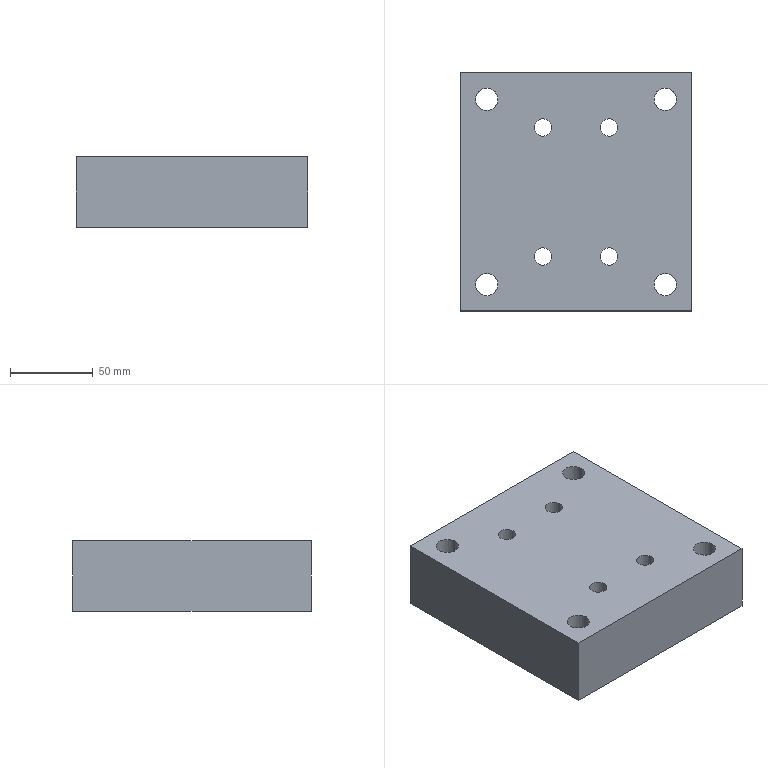Part | STEP file | lll_id2202_x_t | 1 solid | 44 faces | box 140 x 144 x 42.5 mm | volume 713752 mm3 | cylinder 22 | plane 20 | cone 2 | commonest cylinder face diameters 10 x8 10.506 x4 13.509 x4 20.007 x4 10.505 x2
STEP:
#1=CARTESIAN_POINT('',(1650.253,39.,152.5));
#2=VERTEX_POINT('',#1);
#3=CARTESIAN_POINT('',(1645.,39.,152.5));
#4=DIRECTION('',(0.,0.,1.));
#5=DIRECTION('',(1.,0.,0.));
#6=AXIS2_PLACEMENT_3D('',#3,#4,#5);
#7=CIRCLE('',#6,5.253);
#8=EDGE_CURVE('',#2,#2,#7,.T.);
#9=ORIENTED_EDGE('',*,*,#8,.F.);
#10=EDGE_LOOP('',(#9));
#11=FACE_BOUND('',#10,.T.);
#12=CARTESIAN_POINT('',(1610.253,39.,152.5));
#13=VERTEX_POINT('',#12);
#14=CARTESIAN_POINT('',(1605.,39.,152.5));
#15=DIRECTION('',(0.,0.,1.));
#16=DIRECTION('',(1.,0.,0.));
#17=AXIS2_PLACEMENT_3D('',#14,#15,#16);
#18=CIRCLE('',#17,5.253);
#19=EDGE_CURVE('',#13,#13,#18,.T.);
#20=ORIENTED_EDGE('',*,*,#19,.F.);
#21=EDGE_LOOP('',(#20));
#22=FACE_BOUND('',#21,.T.);
#23=CARTESIAN_POINT('',(1610.253,-39.,152.5));
#24=VERTEX_POINT('',#23);
#25=CARTESIAN_POINT('',(1605.,-39.,152.5));
#26=DIRECTION('',(0.,0.,1.));
#27=DIRECTION('',(1.,0.,0.));
#28=AXIS2_PLACEMENT_3D('',#25,#26,#27);
#29=CIRCLE('',#28,5.253);
#30=EDGE_CURVE('',#24,#24,#29,.T.);
#31=ORIENTED_EDGE('',*,*,#30,.F.);
#32=EDGE_LOOP('',(#31));
#33=FACE_BOUND('',#32,.T.);
#34=CARTESIAN_POINT('',(1650.253,-39.,152.5));
#35=VERTEX_POINT('',#34);
#36=CARTESIAN_POINT('',(1645.,-39.,152.5));
#37=DIRECTION('',(0.,0.,1.));
#38=DIRECTION('',(1.,0.,0.));
#39=AXIS2_PLACEMENT_3D('',#36,#37,#38);
#40=CIRCLE('',#39,5.253);
#41=EDGE_CURVE('',#35,#35,#40,.T.);
#42=ORIENTED_EDGE('',*,*,#41,.F.);
#43=EDGE_LOOP('',(#42));
#44=FACE_BOUND('',#43,.T.);
#45=CARTESIAN_POINT('',(1685.755,56.,152.5));
#46=VERTEX_POINT('',#45);
#47=CARTESIAN_POINT('',(1679.,56.,152.5));
#48=DIRECTION('',(0.,0.,1.));
#49=DIRECTION('',(1.,0.,0.));
#50=AXIS2_PLACEMENT_3D('',#47,#48,#49);
#51=CIRCLE('',#50,6.755);
#52=EDGE_CURVE('',#46,#46,#51,.T.);
#53=ORIENTED_EDGE('',*,*,#52,.F.);
#54=EDGE_LOOP('',(#53));
#55=FACE_BOUND('',#54,.T.);
#56=CARTESIAN_POINT('',(1577.755,56.,152.5));
#57=VERTEX_POINT('',#56);
#58=CARTESIAN_POINT('',(1571.,56.,152.5));
#59=DIRECTION('',(0.,0.,1.));
#60=DIRECTION('',(1.,0.,0.));
#61=AXIS2_PLACEMENT_3D('',#58,#59,#60);
#62=CIRCLE('',#61,6.755);
#63=EDGE_CURVE('',#57,#57,#62,.T.);
#64=ORIENTED_EDGE('',*,*,#63,.F.);
#65=EDGE_LOOP('',(#64));
#66=FACE_BOUND('',#65,.T.);
#67=CARTESIAN_POINT('',(1577.755,-56.,152.5));
#68=VERTEX_POINT('',#67);
#69=CARTESIAN_POINT('',(1571.,-56.,152.5));
#70=DIRECTION('',(0.,0.,1.));
#71=DIRECTION('',(1.,0.,0.));
#72=AXIS2_PLACEMENT_3D('',#69,#70,#71);
#73=CIRCLE('',#72,6.755);
#74=EDGE_CURVE('',#68,#68,#73,.T.);
#75=ORIENTED_EDGE('',*,*,#74,.F.);
#76=EDGE_LOOP('',(#75));
#77=FACE_BOUND('',#76,.T.);
#78=CARTESIAN_POINT('',(1685.755,-56.,152.5));
#79=VERTEX_POINT('',#78);
#80=CARTESIAN_POINT('',(1679.,-56.,152.5));
#81=DIRECTION('',(0.,0.,1.));
#82=DIRECTION('',(1.,0.,0.));
#83=AXIS2_PLACEMENT_3D('',#80,#81,#82);
#84=CIRCLE('',#83,6.755);
#85=EDGE_CURVE('',#79,#79,#84,.T.);
#86=ORIENTED_EDGE('',*,*,#85,.F.);
#87=EDGE_LOOP('',(#86));
#88=FACE_BOUND('',#87,.T.);
#89=CARTESIAN_POINT('',(1695.,-72.,152.5));
#90=VERTEX_POINT('',#89);
#91=CARTESIAN_POINT('',(1555.,-72.,152.5));
#92=VERTEX_POINT('',#91);
#93=CARTESIAN_POINT('',(1625.,-72.,152.5));
#94=DIRECTION('',(-1.,0.,0.));
#95=VECTOR('',#94,1.);
#96=LINE('',#93,#95);
#97=EDGE_CURVE('',#90,#92,#96,.T.);
#98=ORIENTED_EDGE('',*,*,#97,.F.);
#99=CARTESIAN_POINT('',(1695.,72.,152.5));
#100=VERTEX_POINT('',#99);
#101=CARTESIAN_POINT('',(1695.,0.,152.5));
#102=DIRECTION('',(0.,-1.,0.));
#103=VECTOR('',#102,1.);
#104=LINE('',#101,#103);
#105=EDGE_CURVE('',#100,#90,#104,.T.);
#106=ORIENTED_EDGE('',*,*,#105,.F.);
#107=CARTESIAN_POINT('',(1555.,72.,152.5));
#108=VERTEX_POINT('',#107);
#109=CARTESIAN_POINT('',(1625.,72.,152.5));
#110=DIRECTION('',(1.,0.,0.));
#111=VECTOR('',#110,1.);
#112=LINE('',#109,#111);
#113=EDGE_CURVE('',#108,#100,#112,.T.);
#114=ORIENTED_EDGE('',*,*,#113,.F.);
#115=CARTESIAN_POINT('',(1555.,0.,152.5));
#116=DIRECTION('',(0.,1.,0.));
#117=VECTOR('',#116,1.);
#118=LINE('',#115,#117);
#119=EDGE_CURVE('',#92,#108,#118,.T.);
#120=ORIENTED_EDGE('',*,*,#119,.F.);
#121=EDGE_LOOP('',(#98,#106,#114,#120));
#122=FACE_BOUND('',#121,.T.);
#123=CARTESIAN_POINT('',(1625.,0.,152.5));
#124=DIRECTION('',(0.,0.,1.));
#125=DIRECTION('',(1.,0.,0.));
#126=AXIS2_PLACEMENT_3D('',#123,#124,#125);
#127=PLANE('',#126);
#128=ADVANCED_FACE('',(#11,#22,#33,#44,#55,#66,#77,#88,#122),#127,.T.);
#129=CARTESIAN_POINT('',(1695.,-72.,110.));
#130=VERTEX_POINT('',#129);
#131=CARTESIAN_POINT('',(1555.,-72.,110.));
#132=VERTEX_POINT('',#131);
#133=CARTESIAN_POINT('',(1625.,-72.,110.));
#134=DIRECTION('',(-1.,0.,0.));
#135=VECTOR('',#134,1.);
#136=LINE('',#133,#135);
#137=EDGE_CURVE('',#130,#132,#136,.T.);
#138=ORIENTED_EDGE('',*,*,#137,.F.);
#139=CARTESIAN_POINT('',(1695.,-72.,-23.));
#140=DIRECTION('',(0.,0.,1.));
#141=VECTOR('',#140,1.);
#142=LINE('',#139,#141);
#143=EDGE_CURVE('',#130,#90,#142,.T.);
#144=ORIENTED_EDGE('',*,*,#143,.T.);
#145=ORIENTED_EDGE('',*,*,#97,.T.);
#146=CARTESIAN_POINT('',(1555.,-72.,-23.));
#147=DIRECTION('',(0.,0.,1.));
#148=VECTOR('',#147,1.);
#149=LINE('',#146,#148);
#150=EDGE_CURVE('',#132,#92,#149,.T.);
#151=ORIENTED_EDGE('',*,*,#150,.F.);
#152=EDGE_LOOP('',(#138,#144,#145,#151));
#153=FACE_OUTER_BOUND('',#152,.T.);
#154=CARTESIAN_POINT('',(1625.,-72.,-23.));
#155=DIRECTION('',(0.,-1.,0.));
#156=DIRECTION('',(0.,0.,-1.));
#157=AXIS2_PLACEMENT_3D('',#154,#155,#156);
#158=PLANE('',#157);
#159=ADVANCED_FACE('',(#153),#158,.T.);
#160=CARTESIAN_POINT('',(1555.,72.,110.));
#161=VERTEX_POINT('',#160);
#162=CARTESIAN_POINT('',(1555.,0.,110.));
#163=DIRECTION('',(0.,-1.,0.));
#164=VECTOR('',#163,1.);
#165=LINE('',#162,#164);
#166=EDGE_CURVE('',#161,#132,#165,.T.);
#167=ORIENTED_EDGE('',*,*,#166,.T.);
#168=ORIENTED_EDGE('',*,*,#150,.T.);
#169=ORIENTED_EDGE('',*,*,#119,.T.);
#170=CARTESIAN_POINT('',(1555.,72.,-23.));
#171=DIRECTION('',(0.,0.,1.));
#172=VECTOR('',#171,1.);
#173=LINE('',#170,#172);
#174=EDGE_CURVE('',#161,#108,#173,.T.);
#175=ORIENTED_EDGE('',*,*,#174,.F.);
#176=EDGE_LOOP('',(#167,#168,#169,#175));
#177=FACE_OUTER_BOUND('',#176,.T.);
#178=CARTESIAN_POINT('',(1555.,0.,-23.));
#179=DIRECTION('',(-1.,0.,0.));
#180=DIRECTION('',(0.,0.,1.));
#181=AXIS2_PLACEMENT_3D('',#178,#179,#180);
#182=PLANE('',#181);
#183=ADVANCED_FACE('',(#177),#182,.T.);
#184=CARTESIAN_POINT('',(1695.,72.,110.));
#185=VERTEX_POINT('',#184);
#186=CARTESIAN_POINT('',(1625.,72.,110.));
#187=DIRECTION('',(1.,0.,0.));
#188=VECTOR('',#187,1.);
#189=LINE('',#186,#188);
#190=EDGE_CURVE('',#161,#185,#189,.T.);
#191=ORIENTED_EDGE('',*,*,#190,.F.);
#192=ORIENTED_EDGE('',*,*,#174,.T.);
#193=ORIENTED_EDGE('',*,*,#113,.T.);
#194=CARTESIAN_POINT('',(1695.,72.,-23.));
#195=DIRECTION('',(0.,0.,1.));
#196=VECTOR('',#195,1.);
#197=LINE('',#194,#196);
#198=EDGE_CURVE('',#185,#100,#197,.T.);
#199=ORIENTED_EDGE('',*,*,#198,.F.);
#200=EDGE_LOOP('',(#191,#192,#193,#199));
#201=FACE_OUTER_BOUND('',#200,.T.);
#202=CARTESIAN_POINT('',(1625.,72.,-23.));
#203=DIRECTION('',(0.,1.,0.));
#204=DIRECTION('',(0.,0.,1.));
#205=AXIS2_PLACEMENT_3D('',#202,#203,#204);
#206=PLANE('',#205);
#207=ADVANCED_FACE('',(#201),#206,.T.);
#208=CARTESIAN_POINT('',(1695.,0.,110.));
#209=DIRECTION('',(0.,-1.,0.));
#210=VECTOR('',#209,1.);
#211=LINE('',#208,#210);
#212=EDGE_CURVE('',#185,#130,#211,.T.);
#213=ORIENTED_EDGE('',*,*,#212,.F.);
#214=ORIENTED_EDGE('',*,*,#198,.T.);
#215=ORIENTED_EDGE('',*,*,#105,.T.);
#216=ORIENTED_EDGE('',*,*,#143,.F.);
#217=EDGE_LOOP('',(#213,#214,#215,#216));
#218=FACE_OUTER_BOUND('',#217,.T.);
#219=CARTESIAN_POINT('',(1695.,0.,-23.));
#220=DIRECTION('',(1.,0.,0.));
#221=DIRECTION('',(0.,0.,-1.));
#222=AXIS2_PLACEMENT_3D('',#219,#220,#221);
#223=PLANE('',#222);
#224=ADVANCED_FACE('',(#218),#223,.T.);
#225=CARTESIAN_POINT('',(1576.253,26.,110.));
#226=VERTEX_POINT('',#225);
#227=CARTESIAN_POINT('',(1571.,26.,110.));
#228=DIRECTION('',(0.,0.,1.));
#229=DIRECTION('',(1.,0.,0.));
#230=AXIS2_PLACEMENT_3D('',#227,#228,#229);
#231=CIRCLE('',#230,5.253);
#232=EDGE_CURVE('',#226,#226,#231,.T.);
#233=ORIENTED_EDGE('',*,*,#232,.T.);
#234=EDGE_LOOP('',(#233));
#235=FACE_BOUND('',#234,.T.);
#236=CARTESIAN_POINT('',(1689.004,56.,110.));
#237=VERTEX_POINT('',#236);
#238=CARTESIAN_POINT('',(1679.,56.,110.));
#239=DIRECTION('',(0.,0.,1.));
#240=DIRECTION('',(1.,0.,0.));
#241=AXIS2_PLACEMENT_3D('',#238,#239,#240);
#242=CIRCLE('',#241,10.004);
#243=EDGE_CURVE('',#237,#237,#242,.T.);
#244=ORIENTED_EDGE('',*,*,#243,.T.);
#245=EDGE_LOOP('',(#244));
#246=FACE_BOUND('',#245,.T.);
#247=CARTESIAN_POINT('',(1581.004,56.,110.));
#248=VERTEX_POINT('',#247);
#249=CARTESIAN_POINT('',(1571.,56.,110.));
#250=DIRECTION('',(0.,0.,1.));
#251=DIRECTION('',(1.,0.,0.));
#252=AXIS2_PLACEMENT_3D('',#249,#250,#251);
#253=CIRCLE('',#252,10.004);
#254=EDGE_CURVE('',#248,#248,#253,.T.);
#255=ORIENTED_EDGE('',*,*,#254,.T.);
#256=EDGE_LOOP('',(#255));
#257=FACE_BOUND('',#256,.T.);
#258=CARTESIAN_POINT('',(1581.004,-56.,110.));
#259=VERTEX_POINT('',#258);
#260=CARTESIAN_POINT('',(1571.,-56.,110.));
#261=DIRECTION('',(0.,0.,1.));
#262=DIRECTION('',(1.,0.,0.));
#263=AXIS2_PLACEMENT_3D('',#260,#261,#262);
#264=CIRCLE('',#263,10.004);
#265=EDGE_CURVE('',#259,#259,#264,.T.);
#266=ORIENTED_EDGE('',*,*,#265,.T.);
#267=EDGE_LOOP('',(#266));
#268=FACE_BOUND('',#267,.T.);
#269=CARTESIAN_POINT('',(1684.253,-26.,110.));
#270=VERTEX_POINT('',#269);
#271=CARTESIAN_POINT('',(1679.,-26.,110.));
#272=DIRECTION('',(0.,0.,1.));
#273=DIRECTION('',(1.,0.,0.));
#274=AXIS2_PLACEMENT_3D('',#271,#272,#273);
#275=CIRCLE('',#274,5.253);
#276=EDGE_CURVE('',#270,#270,#275,.T.);
#277=ORIENTED_EDGE('',*,*,#276,.T.);
#278=EDGE_LOOP('',(#277));
#279=FACE_BOUND('',#278,.T.);
#280=CARTESIAN_POINT('',(1689.004,-56.,110.));
#281=VERTEX_POINT('',#280);
#282=CARTESIAN_POINT('',(1679.,-56.,110.));
#283=DIRECTION('',(0.,0.,1.));
#284=DIRECTION('',(1.,0.,0.));
#285=AXIS2_PLACEMENT_3D('',#282,#283,#284);
#286=CIRCLE('',#285,10.004);
#287=EDGE_CURVE('',#281,#281,#286,.T.);
#288=ORIENTED_EDGE('',*,*,#287,.T.);
#289=EDGE_LOOP('',(#288));
#290=FACE_BOUND('',#289,.T.);
#291=CARTESIAN_POINT('',(1652.051,-11.,110.));
#292=VERTEX_POINT('',#291);
#293=CARTESIAN_POINT('',(1597.949,-11.,110.));
#294=VERTEX_POINT('',#293);
#295=CARTESIAN_POINT('',(2132.435,-11.,110.));
#296=DIRECTION('',(-1.,0.,0.));
#297=VECTOR('',#296,1.);
#298=LINE('',#295,#297);
#299=EDGE_CURVE('',#292,#294,#298,.T.);
#300=ORIENTED_EDGE('',*,*,#299,.T.);
#301=CARTESIAN_POINT('',(1590.,-16.752,110.));
#302=VERTEX_POINT('',#301);
#303=CARTESIAN_POINT('',(1593.408,-13.094,110.));
#304=DIRECTION('',(0.,0.,1.));
#305=DIRECTION('',(1.,0.,0.));
#306=AXIS2_PLACEMENT_3D('',#303,#304,#305);
#307=CIRCLE('',#306,5.);
#308=EDGE_CURVE('',#294,#302,#307,.T.);
#309=ORIENTED_EDGE('',*,*,#308,.T.);
#310=CARTESIAN_POINT('',(1590.,-48.248,110.));
#311=VERTEX_POINT('',#310);
#312=CARTESIAN_POINT('',(1590.,0.,110.));
#313=DIRECTION('',(0.,-1.,0.));
#314=VECTOR('',#313,1.);
#315=LINE('',#312,#314);
#316=EDGE_CURVE('',#302,#311,#315,.T.);
#317=ORIENTED_EDGE('',*,*,#316,.T.);
#318=CARTESIAN_POINT('',(1597.949,-54.,110.));
#319=VERTEX_POINT('',#318);
#320=CARTESIAN_POINT('',(1593.408,-51.906,110.));
#321=DIRECTION('',(0.,0.,1.));
#322=DIRECTION('',(1.,0.,0.));
#323=AXIS2_PLACEMENT_3D('',#320,#321,#322);
#324=CIRCLE('',#323,5.);
#325=EDGE_CURVE('',#311,#319,#324,.T.);
#326=ORIENTED_EDGE('',*,*,#325,.T.);
#327=CARTESIAN_POINT('',(1652.051,-54.,110.));
#328=VERTEX_POINT('',#327);
#329=CARTESIAN_POINT('',(2132.435,-54.,110.));
#330=DIRECTION('',(1.,0.,0.));
#331=VECTOR('',#330,1.);
#332=LINE('',#329,#331);
#333=EDGE_CURVE('',#319,#328,#332,.T.);
#334=ORIENTED_EDGE('',*,*,#333,.T.);
#335=CARTESIAN_POINT('',(1660.,-48.248,110.));
#336=VERTEX_POINT('',#335);
#337=CARTESIAN_POINT('',(1656.592,-51.906,110.));
#338=DIRECTION('',(0.,0.,1.));
#339=DIRECTION('',(1.,0.,0.));
#340=AXIS2_PLACEMENT_3D('',#337,#338,#339);
#341=CIRCLE('',#340,5.);
#342=EDGE_CURVE('',#328,#336,#341,.T.);
#343=ORIENTED_EDGE('',*,*,#342,.T.);
#344=CARTESIAN_POINT('',(1660.,-16.752,110.));
#345=VERTEX_POINT('',#344);
#346=CARTESIAN_POINT('',(1660.,0.,110.));
#347=DIRECTION('',(0.,1.,0.));
#348=VECTOR('',#347,1.);
#349=LINE('',#346,#348);
#350=EDGE_CURVE('',#336,#345,#349,.T.);
#351=ORIENTED_EDGE('',*,*,#350,.T.);
#352=CARTESIAN_POINT('',(1656.592,-13.094,110.));
#353=DIRECTION('',(0.,0.,1.));
#354=DIRECTION('',(1.,0.,0.));
#355=AXIS2_PLACEMENT_3D('',#352,#353,#354);
#356=CIRCLE('',#355,5.);
#357=EDGE_CURVE('',#345,#292,#356,.T.);
#358=ORIENTED_EDGE('',*,*,#357,.T.);
#359=EDGE_LOOP('',(#300,#309,#317,#326,#334,#343,#351,#358));
#360=FACE_BOUND('',#359,.T.);
#361=CARTESIAN_POINT('',(1652.051,54.,110.));
#362=VERTEX_POINT('',#361);
#363=CARTESIAN_POINT('',(1597.949,54.,110.));
#364=VERTEX_POINT('',#363);
#365=CARTESIAN_POINT('',(2132.435,54.,110.));
#366=DIRECTION('',(-1.,0.,0.));
#367=VECTOR('',#366,1.);
#368=LINE('',#365,#367);
#369=EDGE_CURVE('',#362,#364,#368,.T.);
#370=ORIENTED_EDGE('',*,*,#369,.T.);
#371=CARTESIAN_POINT('',(1590.,48.248,110.));
#372=VERTEX_POINT('',#371);
#373=CARTESIAN_POINT('',(1593.408,51.906,110.));
#374=DIRECTION('',(0.,0.,1.));
#375=DIRECTION('',(1.,0.,0.));
#376=AXIS2_PLACEMENT_3D('',#373,#374,#375);
#377=CIRCLE('',#376,5.);
#378=EDGE_CURVE('',#364,#372,#377,.T.);
#379=ORIENTED_EDGE('',*,*,#378,.T.);
#380=CARTESIAN_POINT('',(1590.,16.752,110.));
#381=VERTEX_POINT('',#380);
#382=CARTESIAN_POINT('',(1590.,0.,110.));
#383=DIRECTION('',(0.,-1.,0.));
#384=VECTOR('',#383,1.);
#385=LINE('',#382,#384);
#386=EDGE_CURVE('',#372,#381,#385,.T.);
#387=ORIENTED_EDGE('',*,*,#386,.T.);
#388=CARTESIAN_POINT('',(1597.949,11.,110.));
#389=VERTEX_POINT('',#388);
#390=CARTESIAN_POINT('',(1593.408,13.094,110.));
#391=DIRECTION('',(0.,0.,1.));
#392=DIRECTION('',(1.,0.,0.));
#393=AXIS2_PLACEMENT_3D('',#390,#391,#392);
#394=CIRCLE('',#393,5.);
#395=EDGE_CURVE('',#381,#389,#394,.T.);
#396=ORIENTED_EDGE('',*,*,#395,.T.);
#397=CARTESIAN_POINT('',(1652.051,11.,110.));
#398=VERTEX_POINT('',#397);
#399=CARTESIAN_POINT('',(2132.435,11.,110.));
#400=DIRECTION('',(1.,0.,0.));
#401=VECTOR('',#400,1.);
#402=LINE('',#399,#401);
#403=EDGE_CURVE('',#389,#398,#402,.T.);
#404=ORIENTED_EDGE('',*,*,#403,.T.);
#405=CARTESIAN_POINT('',(1660.,16.752,110.));
#406=VERTEX_POINT('',#405);
#407=CARTESIAN_POINT('',(1656.592,13.094,110.));
#408=DIRECTION('',(0.,0.,1.));
#409=DIRECTION('',(1.,0.,0.));
#410=AXIS2_PLACEMENT_3D('',#407,#408,#409);
#411=CIRCLE('',#410,5.);
#412=EDGE_CURVE('',#398,#406,#411,.T.);
#413=ORIENTED_EDGE('',*,*,#412,.T.);
#414=CARTESIAN_POINT('',(1660.,48.248,110.));
#415=VERTEX_POINT('',#414);
#416=CARTESIAN_POINT('',(1660.,0.,110.));
#417=DIRECTION('',(0.,1.,0.));
#418=VECTOR('',#417,1.);
#419=LINE('',#416,#418);
#420=EDGE_CURVE('',#406,#415,#419,.T.);
#421=ORIENTED_EDGE('',*,*,#420,.T.);
#422=CARTESIAN_POINT('',(1656.592,51.906,110.));
#423=DIRECTION('',(0.,0.,1.));
#424=DIRECTION('',(1.,0.,0.));
#425=AXIS2_PLACEMENT_3D('',#422,#423,#424);
#426=CIRCLE('',#425,5.);
#427=EDGE_CURVE('',#415,#362,#426,.T.);
#428=ORIENTED_EDGE('',*,*,#427,.T.);
#429=EDGE_LOOP('',(#370,#379,#387,#396,#404,#413,#421,#428));
#430=FACE_BOUND('',#429,.T.);
#431=ORIENTED_EDGE('',*,*,#137,.T.);
#432=ORIENTED_EDGE('',*,*,#166,.F.);
#433=ORIENTED_EDGE('',*,*,#190,.T.);
#434=ORIENTED_EDGE('',*,*,#212,.T.);
#435=EDGE_LOOP('',(#431,#432,#433,#434));
#436=FACE_BOUND('',#435,.T.);
#437=CARTESIAN_POINT('',(2132.435,0.,110.));
#438=DIRECTION('',(0.,0.,1.));
#439=DIRECTION('',(1.,0.,0.));
#440=AXIS2_PLACEMENT_3D('',#437,#438,#439);
#441=PLANE('',#440);
#442=ADVANCED_FACE('',(#235,#246,#257,#268,#279,#290,#360,#430,#436),#441,.F.);
#443=CARTESIAN_POINT('',(1597.949,11.,125.));
#444=VERTEX_POINT('',#443);
#445=CARTESIAN_POINT('',(1597.949,11.,125.));
#446=DIRECTION('',(0.,0.,-1.));
#447=VECTOR('',#446,1.);
#448=LINE('',#445,#447);
#449=EDGE_CURVE('',#444,#389,#448,.T.);
#450=ORIENTED_EDGE('',*,*,#449,.F.);
#451=CARTESIAN_POINT('',(1652.051,11.,125.));
#452=VERTEX_POINT('',#451);
#453=CARTESIAN_POINT('',(1625.,11.,125.));
#454=DIRECTION('',(1.,0.,0.));
#455=VECTOR('',#454,1.);
#456=LINE('',#453,#455);
#457=EDGE_CURVE('',#444,#452,#456,.T.);
#458=ORIENTED_EDGE('',*,*,#457,.T.);
#459=CARTESIAN_POINT('',(1652.051,11.,125.));
#460=DIRECTION('',(0.,0.,1.));
#461=VECTOR('',#460,1.);
#462=LINE('',#459,#461);
#463=EDGE_CURVE('',#398,#452,#462,.T.);
#464=ORIENTED_EDGE('',*,*,#463,.F.);
#465=ORIENTED_EDGE('',*,*,#403,.F.);
#466=EDGE_LOOP('',(#450,#458,#464,#465));
#467=FACE_OUTER_BOUND('',#466,.T.);
#468=CARTESIAN_POINT('',(1625.,11.,-23.));
#469=DIRECTION('',(0.,-1.,0.));
#470=DIRECTION('',(0.,0.,-1.));
#471=AXIS2_PLACEMENT_3D('',#468,#469,#470);
#472=PLANE('',#471);
#473=ADVANCED_FACE('',(#467),#472,.F.);
#474=CARTESIAN_POINT('',(1590.,48.248,125.));
#475=VERTEX_POINT('',#474);
#476=CARTESIAN_POINT('',(1590.,48.248,125.));
#477=DIRECTION('',(0.,0.,-1.));
#478=VECTOR('',#477,1.);
#479=LINE('',#476,#478);
#480=EDGE_CURVE('',#475,#372,#479,.T.);
#481=ORIENTED_EDGE('',*,*,#480,.F.);
#482=CARTESIAN_POINT('',(1590.,16.752,125.));
#483=VERTEX_POINT('',#482);
#484=CARTESIAN_POINT('',(1590.,32.5,125.));
#485=DIRECTION('',(0.,-1.,0.));
#486=VECTOR('',#485,1.);
#487=LINE('',#484,#486);
#488=EDGE_CURVE('',#475,#483,#487,.T.);
#489=ORIENTED_EDGE('',*,*,#488,.T.);
#490=CARTESIAN_POINT('',(1590.,16.752,125.));
#491=DIRECTION('',(0.,0.,1.));
#492=VECTOR('',#491,1.);
#493=LINE('',#490,#492);
#494=EDGE_CURVE('',#381,#483,#493,.T.);
#495=ORIENTED_EDGE('',*,*,#494,.F.);
#496=ORIENTED_EDGE('',*,*,#386,.F.);
#497=EDGE_LOOP('',(#481,#489,#495,#496));
#498=FACE_OUTER_BOUND('',#497,.T.);
#499=CARTESIAN_POINT('',(1590.,32.5,-23.));
#500=DIRECTION('',(-1.,0.,0.));
#501=DIRECTION('',(0.,0.,1.));
#502=AXIS2_PLACEMENT_3D('',#499,#500,#501);
#503=PLANE('',#502);
#504=ADVANCED_FACE('',(#498),#503,.F.);
#505=CARTESIAN_POINT('',(1652.051,54.,125.));
#506=VERTEX_POINT('',#505);
#507=CARTESIAN_POINT('',(1652.051,54.,125.));
#508=DIRECTION('',(0.,0.,-1.));
#509=VECTOR('',#508,1.);
#510=LINE('',#507,#509);
#511=EDGE_CURVE('',#506,#362,#510,.T.);
#512=ORIENTED_EDGE('',*,*,#511,.F.);
#513=CARTESIAN_POINT('',(1597.949,54.,125.));
#514=VERTEX_POINT('',#513);
#515=CARTESIAN_POINT('',(1625.,54.,125.));
#516=DIRECTION('',(-1.,0.,0.));
#517=VECTOR('',#516,1.);
#518=LINE('',#515,#517);
#519=EDGE_CURVE('',#506,#514,#518,.T.);
#520=ORIENTED_EDGE('',*,*,#519,.T.);
#521=CARTESIAN_POINT('',(1597.949,54.,125.));
#522=DIRECTION('',(0.,0.,1.));
#523=VECTOR('',#522,1.);
#524=LINE('',#521,#523);
#525=EDGE_CURVE('',#364,#514,#524,.T.);
#526=ORIENTED_EDGE('',*,*,#525,.F.);
#527=ORIENTED_EDGE('',*,*,#369,.F.);
#528=EDGE_LOOP('',(#512,#520,#526,#527));
#529=FACE_OUTER_BOUND('',#528,.T.);
#530=CARTESIAN_POINT('',(1625.,54.,-23.));
#531=DIRECTION('',(0.,1.,0.));
#532=DIRECTION('',(0.,0.,1.));
#533=AXIS2_PLACEMENT_3D('',#530,#531,#532);
#534=PLANE('',#533);
#535=ADVANCED_FACE('',(#529),#534,.F.);
#536=CARTESIAN_POINT('',(1660.,16.752,125.));
#537=VERTEX_POINT('',#536);
#538=CARTESIAN_POINT('',(1660.,16.752,125.));
#539=DIRECTION('',(0.,0.,-1.));
#540=VECTOR('',#539,1.);
#541=LINE('',#538,#540);
#542=EDGE_CURVE('',#537,#406,#541,.T.);
#543=ORIENTED_EDGE('',*,*,#542,.F.);
#544=CARTESIAN_POINT('',(1660.,48.248,125.));
#545=VERTEX_POINT('',#544);
#546=CARTESIAN_POINT('',(1660.,32.5,125.));
#547=DIRECTION('',(0.,1.,0.));
#548=VECTOR('',#547,1.);
#549=LINE('',#546,#548);
#550=EDGE_CURVE('',#537,#545,#549,.T.);
#551=ORIENTED_EDGE('',*,*,#550,.T.);
#552=CARTESIAN_POINT('',(1660.,48.248,125.));
#553=DIRECTION('',(0.,0.,1.));
#554=VECTOR('',#553,1.);
#555=LINE('',#552,#554);
#556=EDGE_CURVE('',#415,#545,#555,.T.);
#557=ORIENTED_EDGE('',*,*,#556,.F.);
#558=ORIENTED_EDGE('',*,*,#420,.F.);
#559=EDGE_LOOP('',(#543,#551,#557,#558));
#560=FACE_OUTER_BOUND('',#559,.T.);
#561=CARTESIAN_POINT('',(1660.,32.5,-23.));
#562=DIRECTION('',(1.,0.,0.));
#563=DIRECTION('',(0.,0.,-1.));
#564=AXIS2_PLACEMENT_3D('',#561,#562,#563);
#565=PLANE('',#564);
#566=ADVANCED_FACE('',(#560),#565,.F.);
#567=ORIENTED_EDGE('',*,*,#494,.T.);
#568=CARTESIAN_POINT('',(1593.408,13.094,125.));
#569=DIRECTION('',(0.,0.,1.));
#570=DIRECTION('',(1.,0.,0.));
#571=AXIS2_PLACEMENT_3D('',#568,#569,#570);
#572=CIRCLE('',#571,5.);
#573=EDGE_CURVE('',#483,#444,#572,.T.);
#574=ORIENTED_EDGE('',*,*,#573,.T.);
#575=ORIENTED_EDGE('',*,*,#449,.T.);
#576=ORIENTED_EDGE('',*,*,#395,.F.);
#577=EDGE_LOOP('',(#567,#574,#575,#576));
#578=FACE_OUTER_BOUND('',#577,.T.);
#579=CARTESIAN_POINT('',(1593.408,13.094,125.));
#580=DIRECTION('',(0.,0.,-1.));
#581=DIRECTION('',(1.,0.,0.));
#582=AXIS2_PLACEMENT_3D('',#579,#580,#581);
#583=CYLINDRICAL_SURFACE('',#582,5.);
#584=ADVANCED_FACE('',(#578),#583,.F.);
#585=ORIENTED_EDGE('',*,*,#556,.T.);
#586=CARTESIAN_POINT('',(1656.592,51.906,125.));
#587=DIRECTION('',(0.,0.,1.));
#588=DIRECTION('',(1.,0.,0.));
#589=AXIS2_PLACEMENT_3D('',#586,#587,#588);
#590=CIRCLE('',#589,5.);
#591=EDGE_CURVE('',#545,#506,#590,.T.);
#592=ORIENTED_EDGE('',*,*,#591,.T.);
#593=ORIENTED_EDGE('',*,*,#511,.T.);
#594=ORIENTED_EDGE('',*,*,#427,.F.);
#595=EDGE_LOOP('',(#585,#592,#593,#594));
#596=FACE_OUTER_BOUND('',#595,.T.);
#597=CARTESIAN_POINT('',(1656.592,51.906,125.));
#598=DIRECTION('',(0.,0.,-1.));
#599=DIRECTION('',(1.,0.,0.));
#600=AXIS2_PLACEMENT_3D('',#597,#598,#599);
#601=CYLINDRICAL_SURFACE('',#600,5.);
#602=ADVANCED_FACE('',(#596),#601,.F.);
#603=ORIENTED_EDGE('',*,*,#525,.T.);
#604=CARTESIAN_POINT('',(1593.408,51.906,125.));
#605=DIRECTION('',(0.,0.,1.));
#606=DIRECTION('',(1.,0.,0.));
#607=AXIS2_PLACEMENT_3D('',#604,#605,#606);
#608=CIRCLE('',#607,5.);
#609=EDGE_CURVE('',#514,#475,#608,.T.);
#610=ORIENTED_EDGE('',*,*,#609,.T.);
#611=ORIENTED_EDGE('',*,*,#480,.T.);
#612=ORIENTED_EDGE('',*,*,#378,.F.);
#613=EDGE_LOOP('',(#603,#610,#611,#612));
#614=FACE_OUTER_BOUND('',#613,.T.);
#615=CARTESIAN_POINT('',(1593.408,51.906,125.));
#616=DIRECTION('',(0.,0.,-1.));
#617=DIRECTION('',(1.,0.,0.));
#618=AXIS2_PLACEMENT_3D('',#615,#616,#617);
#619=CYLINDRICAL_SURFACE('',#618,5.);
#620=ADVANCED_FACE('',(#614),#619,.F.);
#621=ORIENTED_EDGE('',*,*,#463,.T.);
#622=CARTESIAN_POINT('',(1656.592,13.094,125.));
#623=DIRECTION('',(0.,0.,1.));
#624=DIRECTION('',(1.,0.,0.));
#625=AXIS2_PLACEMENT_3D('',#622,#623,#624);
#626=CIRCLE('',#625,5.);
#627=EDGE_CURVE('',#452,#537,#626,.T.);
#628=ORIENTED_EDGE('',*,*,#627,.T.);
#629=ORIENTED_EDGE('',*,*,#542,.T.);
#630=ORIENTED_EDGE('',*,*,#412,.F.);
#631=EDGE_LOOP('',(#621,#628,#629,#630));
#632=FACE_OUTER_BOUND('',#631,.T.);
#633=CARTESIAN_POINT('',(1656.592,13.094,125.));
#634=DIRECTION('',(0.,0.,-1.));
#635=DIRECTION('',(1.,0.,0.));
#636=AXIS2_PLACEMENT_3D('',#633,#634,#635);
#637=CYLINDRICAL_SURFACE('',#636,5.);
#638=ADVANCED_FACE('',(#632),#637,.F.);
#639=CARTESIAN_POINT('',(1650.253,39.,125.));
#640=VERTEX_POINT('',#639);
#641=CARTESIAN_POINT('',(1645.,39.,125.));
#642=DIRECTION('',(0.,0.,1.));
#643=DIRECTION('',(1.,0.,0.));
#644=AXIS2_PLACEMENT_3D('',#641,#642,#643);
#645=CIRCLE('',#644,5.253);
#646=EDGE_CURVE('',#640,#640,#645,.T.);
#647=ORIENTED_EDGE('',*,*,#646,.T.);
#648=EDGE_LOOP('',(#647));
#649=FACE_BOUND('',#648,.T.);
#650=CARTESIAN_POINT('',(1610.253,39.,125.));
#651=VERTEX_POINT('',#650);
#652=CARTESIAN_POINT('',(1605.,39.,125.));
#653=DIRECTION('',(0.,0.,1.));
#654=DIRECTION('',(1.,0.,0.));
#655=AXIS2_PLACEMENT_3D('',#652,#653,#654);
#656=CIRCLE('',#655,5.253);
#657=EDGE_CURVE('',#651,#651,#656,.T.);
#658=ORIENTED_EDGE('',*,*,#657,.T.);
#659=EDGE_LOOP('',(#658));
#660=FACE_BOUND('',#659,.T.);
#661=ORIENTED_EDGE('',*,*,#457,.F.);
#662=ORIENTED_EDGE('',*,*,#573,.F.);
#663=ORIENTED_EDGE('',*,*,#488,.F.);
#664=ORIENTED_EDGE('',*,*,#609,.F.);
#665=ORIENTED_EDGE('',*,*,#519,.F.);
#666=ORIENTED_EDGE('',*,*,#591,.F.);
#667=ORIENTED_EDGE('',*,*,#550,.F.);
#668=ORIENTED_EDGE('',*,*,#627,.F.);
#669=EDGE_LOOP('',(#661,#662,#663,#664,#665,#666,#667,#668));
#670=FACE_BOUND('',#669,.T.);
#671=CARTESIAN_POINT('',(1625.,32.5,125.));
#672=DIRECTION('',(0.,0.,1.));
#673=DIRECTION('',(1.,0.,0.));
#674=AXIS2_PLACEMENT_3D('',#671,#672,#673);
#675=PLANE('',#674);
#676=ADVANCED_FACE('',(#649,#660,#670),#675,.F.);
#677=CARTESIAN_POINT('',(1597.949,-54.,125.));
#678=VERTEX_POINT('',#677);
#679=CARTESIAN_POINT('',(1597.949,-54.,125.));
#680=DIRECTION('',(0.,0.,-1.));
#681=VECTOR('',#680,1.);
#682=LINE('',#679,#681);
#683=EDGE_CURVE('',#678,#319,#682,.T.);
#684=ORIENTED_EDGE('',*,*,#683,.F.);
#685=CARTESIAN_POINT('',(1652.051,-54.,125.));
#686=VERTEX_POINT('',#685);
#687=CARTESIAN_POINT('',(1625.,-54.,125.));
#688=DIRECTION('',(1.,0.,0.));
#689=VECTOR('',#688,1.);
#690=LINE('',#687,#689);
#691=EDGE_CURVE('',#678,#686,#690,.T.);
#692=ORIENTED_EDGE('',*,*,#691,.T.);
#693=CARTESIAN_POINT('',(1652.051,-54.,125.));
#694=DIRECTION('',(0.,0.,1.));
#695=VECTOR('',#694,1.);
#696=LINE('',#693,#695);
#697=EDGE_CURVE('',#328,#686,#696,.T.);
#698=ORIENTED_EDGE('',*,*,#697,.F.);
#699=ORIENTED_EDGE('',*,*,#333,.F.);
#700=EDGE_LOOP('',(#684,#692,#698,#699));
#701=FACE_OUTER_BOUND('',#700,.T.);
#702=CARTESIAN_POINT('',(1625.,-54.,-23.));
#703=DIRECTION('',(0.,-1.,0.));
#704=DIRECTION('',(0.,0.,-1.));
#705=AXIS2_PLACEMENT_3D('',#702,#703,#704);
#706=PLANE('',#705);
#707=ADVANCED_FACE('',(#701),#706,.F.);
#708=CARTESIAN_POINT('',(1590.,-16.752,125.));
#709=VERTEX_POINT('',#708);
#710=CARTESIAN_POINT('',(1590.,-16.752,125.));
#711=DIRECTION('',(0.,0.,-1.));
#712=VECTOR('',#711,1.);
#713=LINE('',#710,#712);
#714=EDGE_CURVE('',#709,#302,#713,.T.);
#715=ORIENTED_EDGE('',*,*,#714,.F.);
#716=CARTESIAN_POINT('',(1590.,-48.248,125.));
#717=VERTEX_POINT('',#716);
#718=CARTESIAN_POINT('',(1590.,-32.5,125.));
#719=DIRECTION('',(0.,-1.,0.));
#720=VECTOR('',#719,1.);
#721=LINE('',#718,#720);
#722=EDGE_CURVE('',#709,#717,#721,.T.);
#723=ORIENTED_EDGE('',*,*,#722,.T.);
#724=CARTESIAN_POINT('',(1590.,-48.248,125.));
#725=DIRECTION('',(0.,0.,1.));
#726=VECTOR('',#725,1.);
#727=LINE('',#724,#726);
#728=EDGE_CURVE('',#311,#717,#727,.T.);
#729=ORIENTED_EDGE('',*,*,#728,.F.);
#730=ORIENTED_EDGE('',*,*,#316,.F.);
#731=EDGE_LOOP('',(#715,#723,#729,#730));
#732=FACE_OUTER_BOUND('',#731,.T.);
#733=CARTESIAN_POINT('',(1590.,-32.5,-23.));
#734=DIRECTION('',(-1.,0.,0.));
#735=DIRECTION('',(0.,0.,1.));
#736=AXIS2_PLACEMENT_3D('',#733,#734,#735);
#737=PLANE('',#736);
#738=ADVANCED_FACE('',(#732),#737,.F.);
#739=CARTESIAN_POINT('',(1652.051,-11.,125.));
#740=VERTEX_POINT('',#739);
#741=CARTESIAN_POINT('',(1652.051,-11.,125.));
#742=DIRECTION('',(0.,0.,-1.));
#743=VECTOR('',#742,1.);
#744=LINE('',#741,#743);
#745=EDGE_CURVE('',#740,#292,#744,.T.);
#746=ORIENTED_EDGE('',*,*,#745,.F.);
#747=CARTESIAN_POINT('',(1597.949,-11.,125.));
#748=VERTEX_POINT('',#747);
#749=CARTESIAN_POINT('',(1625.,-11.,125.));
#750=DIRECTION('',(-1.,0.,0.));
#751=VECTOR('',#750,1.);
#752=LINE('',#749,#751);
#753=EDGE_CURVE('',#740,#748,#752,.T.);
#754=ORIENTED_EDGE('',*,*,#753,.T.);
#755=CARTESIAN_POINT('',(1597.949,-11.,125.));
#756=DIRECTION('',(0.,0.,1.));
#757=VECTOR('',#756,1.);
#758=LINE('',#755,#757);
#759=EDGE_CURVE('',#294,#748,#758,.T.);
#760=ORIENTED_EDGE('',*,*,#759,.F.);
#761=ORIENTED_EDGE('',*,*,#299,.F.);
#762=EDGE_LOOP('',(#746,#754,#760,#761));
#763=FACE_OUTER_BOUND('',#762,.T.);
#764=CARTESIAN_POINT('',(1625.,-11.,-23.));
#765=DIRECTION('',(0.,1.,0.));
#766=DIRECTION('',(0.,0.,1.));
#767=AXIS2_PLACEMENT_3D('',#764,#765,#766);
#768=PLANE('',#767);
#769=ADVANCED_FACE('',(#763),#768,.F.);
#770=CARTESIAN_POINT('',(1660.,-48.248,125.));
#771=VERTEX_POINT('',#770);
#772=CARTESIAN_POINT('',(1660.,-48.248,125.));
#773=DIRECTION('',(0.,0.,-1.));
#774=VECTOR('',#773,1.);
#775=LINE('',#772,#774);
#776=EDGE_CURVE('',#771,#336,#775,.T.);
#777=ORIENTED_EDGE('',*,*,#776,.F.);
#778=CARTESIAN_POINT('',(1660.,-16.752,125.));
#779=VERTEX_POINT('',#778);
#780=CARTESIAN_POINT('',(1660.,-32.5,125.));
#781=DIRECTION('',(0.,1.,0.));
#782=VECTOR('',#781,1.);
#783=LINE('',#780,#782);
#784=EDGE_CURVE('',#771,#779,#783,.T.);
#785=ORIENTED_EDGE('',*,*,#784,.T.);
#786=CARTESIAN_POINT('',(1660.,-16.752,125.));
#787=DIRECTION('',(0.,0.,1.));
#788=VECTOR('',#787,1.);
#789=LINE('',#786,#788);
#790=EDGE_CURVE('',#345,#779,#789,.T.);
#791=ORIENTED_EDGE('',*,*,#790,.F.);
#792=ORIENTED_EDGE('',*,*,#350,.F.);
#793=EDGE_LOOP('',(#777,#785,#791,#792));
#794=FACE_OUTER_BOUND('',#793,.T.);
#795=CARTESIAN_POINT('',(1660.,-32.5,-23.));
#796=DIRECTION('',(1.,0.,0.));
#797=DIRECTION('',(0.,0.,-1.));
#798=AXIS2_PLACEMENT_3D('',#795,#796,#797);
#799=PLANE('',#798);
#800=ADVANCED_FACE('',(#794),#799,.F.);
#801=ORIENTED_EDGE('',*,*,#728,.T.);
#802=CARTESIAN_POINT('',(1593.408,-51.906,125.));
#803=DIRECTION('',(0.,0.,1.));
#804=DIRECTION('',(1.,0.,0.));
#805=AXIS2_PLACEMENT_3D('',#802,#803,#804);
#806=CIRCLE('',#805,5.);
#807=EDGE_CURVE('',#717,#678,#806,.T.);
#808=ORIENTED_EDGE('',*,*,#807,.T.);
#809=ORIENTED_EDGE('',*,*,#683,.T.);
#810=ORIENTED_EDGE('',*,*,#325,.F.);
#811=EDGE_LOOP('',(#801,#808,#809,#810));
#812=FACE_OUTER_BOUND('',#811,.T.);
#813=CARTESIAN_POINT('',(1593.408,-51.906,125.));
#814=DIRECTION('',(0.,0.,-1.));
#815=DIRECTION('',(1.,0.,0.));
#816=AXIS2_PLACEMENT_3D('',#813,#814,#815);
#817=CYLINDRICAL_SURFACE('',#816,5.);
#818=ADVANCED_FACE('',(#812),#817,.F.);
#819=ORIENTED_EDGE('',*,*,#790,.T.);
#820=CARTESIAN_POINT('',(1656.592,-13.094,125.));
#821=DIRECTION('',(0.,0.,1.));
#822=DIRECTION('',(1.,0.,0.));
#823=AXIS2_PLACEMENT_3D('',#820,#821,#822);
#824=CIRCLE('',#823,5.);
#825=EDGE_CURVE('',#779,#740,#824,.T.);
#826=ORIENTED_EDGE('',*,*,#825,.T.);
#827=ORIENTED_EDGE('',*,*,#745,.T.);
#828=ORIENTED_EDGE('',*,*,#357,.F.);
#829=EDGE_LOOP('',(#819,#826,#827,#828));
#830=FACE_OUTER_BOUND('',#829,.T.);
#831=CARTESIAN_POINT('',(1656.592,-13.094,125.));
#832=DIRECTION('',(0.,0.,-1.));
#833=DIRECTION('',(1.,0.,0.));
#834=AXIS2_PLACEMENT_3D('',#831,#832,#833);
#835=CYLINDRICAL_SURFACE('',#834,5.);
#836=ADVANCED_FACE('',(#830),#835,.F.);
#837=ORIENTED_EDGE('',*,*,#759,.T.);
#838=CARTESIAN_POINT('',(1593.408,-13.094,125.));
#839=DIRECTION('',(0.,0.,1.));
#840=DIRECTION('',(1.,0.,0.));
#841=AXIS2_PLACEMENT_3D('',#838,#839,#840);
#842=CIRCLE('',#841,5.);
#843=EDGE_CURVE('',#748,#709,#842,.T.);
#844=ORIENTED_EDGE('',*,*,#843,.T.);
#845=ORIENTED_EDGE('',*,*,#714,.T.);
#846=ORIENTED_EDGE('',*,*,#308,.F.);
#847=EDGE_LOOP('',(#837,#844,#845,#846));
#848=FACE_OUTER_BOUND('',#847,.T.);
#849=CARTESIAN_POINT('',(1593.408,-13.094,125.));
#850=DIRECTION('',(0.,0.,-1.));
#851=DIRECTION('',(1.,0.,0.));
#852=AXIS2_PLACEMENT_3D('',#849,#850,#851);
#853=CYLINDRICAL_SURFACE('',#852,5.);
#854=ADVANCED_FACE('',(#848),#853,.F.);
#855=ORIENTED_EDGE('',*,*,#697,.T.);
#856=CARTESIAN_POINT('',(1656.592,-51.906,125.));
#857=DIRECTION('',(0.,0.,1.));
#858=DIRECTION('',(1.,0.,0.));
#859=AXIS2_PLACEMENT_3D('',#856,#857,#858);
#860=CIRCLE('',#859,5.);
#861=EDGE_CURVE('',#686,#771,#860,.T.);
#862=ORIENTED_EDGE('',*,*,#861,.T.);
#863=ORIENTED_EDGE('',*,*,#776,.T.);
#864=ORIENTED_EDGE('',*,*,#342,.F.);
#865=EDGE_LOOP('',(#855,#862,#863,#864));
#866=FACE_OUTER_BOUND('',#865,.T.);
#867=CARTESIAN_POINT('',(1656.592,-51.906,125.));
#868=DIRECTION('',(0.,0.,-1.));
#869=DIRECTION('',(1.,0.,0.));
#870=AXIS2_PLACEMENT_3D('',#867,#868,#869);
#871=CYLINDRICAL_SURFACE('',#870,5.);
#872=ADVANCED_FACE('',(#866),#871,.F.);
#873=CARTESIAN_POINT('',(1610.253,-39.,125.));
#874=VERTEX_POINT('',#873);
#875=CARTESIAN_POINT('',(1605.,-39.,125.));
#876=DIRECTION('',(0.,0.,1.));
#877=DIRECTION('',(1.,0.,0.));
#878=AXIS2_PLACEMENT_3D('',#875,#876,#877);
#879=CIRCLE('',#878,5.253);
#880=EDGE_CURVE('',#874,#874,#879,.T.);
#881=ORIENTED_EDGE('',*,*,#880,.T.);
#882=EDGE_LOOP('',(#881));
#883=FACE_BOUND('',#882,.T.);
#884=CARTESIAN_POINT('',(1650.253,-39.,125.));
#885=VERTEX_POINT('',#884);
#886=CARTESIAN_POINT('',(1645.,-39.,125.));
#887=DIRECTION('',(0.,0.,1.));
#888=DIRECTION('',(1.,0.,0.));
#889=AXIS2_PLACEMENT_3D('',#886,#887,#888);
#890=CIRCLE('',#889,5.253);
#891=EDGE_CURVE('',#885,#885,#890,.T.);
#892=ORIENTED_EDGE('',*,*,#891,.T.);
#893=EDGE_LOOP('',(#892));
#894=FACE_BOUND('',#893,.T.);
#895=ORIENTED_EDGE('',*,*,#691,.F.);
#896=ORIENTED_EDGE('',*,*,#807,.F.);
#897=ORIENTED_EDGE('',*,*,#722,.F.);
#898=ORIENTED_EDGE('',*,*,#843,.F.);
#899=ORIENTED_EDGE('',*,*,#753,.F.);
#900=ORIENTED_EDGE('',*,*,#825,.F.);
#901=ORIENTED_EDGE('',*,*,#784,.F.);
#902=ORIENTED_EDGE('',*,*,#861,.F.);
#903=EDGE_LOOP('',(#895,#896,#897,#898,#899,#900,#901,#902));
#904=FACE_BOUND('',#903,.T.);
#905=CARTESIAN_POINT('',(1625.,-32.5,125.));
#906=DIRECTION('',(0.,0.,1.));
#907=DIRECTION('',(1.,0.,0.));
#908=AXIS2_PLACEMENT_3D('',#905,#906,#907);
#909=PLANE('',#908);
#910=ADVANCED_FACE('',(#883,#894,#904),#909,.F.);
#911=ORIENTED_EDGE('',*,*,#85,.T.);
#912=EDGE_LOOP('',(#911));
#913=FACE_BOUND('',#912,.T.);
#914=CARTESIAN_POINT('',(1685.755,-56.,125.));
#915=VERTEX_POINT('',#914);
#916=CARTESIAN_POINT('',(1679.,-56.,125.));
#917=DIRECTION('',(0.,0.,1.));
#918=DIRECTION('',(1.,0.,0.));
#919=AXIS2_PLACEMENT_3D('',#916,#917,#918);
#920=CIRCLE('',#919,6.755);
#921=EDGE_CURVE('',#915,#915,#920,.T.);
#922=ORIENTED_EDGE('',*,*,#921,.F.);
#923=EDGE_LOOP('',(#922));
#924=FACE_BOUND('',#923,.T.);
#925=CARTESIAN_POINT('',(1679.,-56.,105.));
#926=DIRECTION('',(0.,0.,1.));
#927=DIRECTION('',(1.,0.,0.));
#928=AXIS2_PLACEMENT_3D('',#925,#926,#927);
#929=CYLINDRICAL_SURFACE('',#928,6.755);
#930=ADVANCED_FACE('',(#913,#924),#929,.F.);
#931=ORIENTED_EDGE('',*,*,#921,.T.);
#932=EDGE_LOOP('',(#931));
#933=FACE_BOUND('',#932,.T.);
#934=CARTESIAN_POINT('',(1689.004,-56.,125.));
#935=VERTEX_POINT('',#934);
#936=CARTESIAN_POINT('',(1679.,-56.,125.));
#937=DIRECTION('',(0.,0.,1.));
#938=DIRECTION('',(1.,0.,0.));
#939=AXIS2_PLACEMENT_3D('',#936,#937,#938);
#940=CIRCLE('',#939,10.004);
#941=EDGE_CURVE('',#935,#935,#940,.T.);
#942=ORIENTED_EDGE('',*,*,#941,.F.);
#943=EDGE_LOOP('',(#942));
#944=FACE_BOUND('',#943,.T.);
#945=CARTESIAN_POINT('',(1679.,-56.,125.));
#946=DIRECTION('',(0.,0.,1.));
#947=DIRECTION('',(1.,0.,0.));
#948=AXIS2_PLACEMENT_3D('',#945,#946,#947);
#949=PLANE('',#948);
#950=ADVANCED_FACE('',(#933,#944),#949,.F.);
#951=ORIENTED_EDGE('',*,*,#941,.T.);
#952=EDGE_LOOP('',(#951));
#953=FACE_BOUND('',#952,.T.);
#954=ORIENTED_EDGE('',*,*,#287,.F.);
#955=EDGE_LOOP('',(#954));
#956=FACE_BOUND('',#955,.T.);
#957=CARTESIAN_POINT('',(1679.,-56.,110.));
#958=DIRECTION('',(0.,0.,1.));
#959=DIRECTION('',(1.,0.,0.));
#960=AXIS2_PLACEMENT_3D('',#957,#958,#959);
#961=CYLINDRICAL_SURFACE('',#960,10.004);
#962=ADVANCED_FACE('',(#953,#956),#961,.F.);
#963=CARTESIAN_POINT('',(1684.253,-26.,139.754));
#964=VERTEX_POINT('',#963);
#965=CARTESIAN_POINT('',(1679.,-26.,139.754));
#966=DIRECTION('',(0.,0.,1.));
#967=DIRECTION('',(1.,0.,0.));
#968=AXIS2_PLACEMENT_3D('',#965,#966,#967);
#969=CIRCLE('',#968,5.253);
#970=EDGE_CURVE('',#964,#964,#969,.T.);
#971=ORIENTED_EDGE('',*,*,#970,.T.);
#972=EDGE_LOOP('',(#971));
#973=FACE_BOUND('',#972,.T.);
#974=ORIENTED_EDGE('',*,*,#276,.F.);
#975=EDGE_LOOP('',(#974));
#976=FACE_BOUND('',#975,.T.);
#977=CARTESIAN_POINT('',(1679.,-26.,105.));
#978=DIRECTION('',(0.,0.,1.));
#979=DIRECTION('',(1.,0.,0.));
#980=AXIS2_PLACEMENT_3D('',#977,#978,#979);
#981=CYLINDRICAL_SURFACE('',#980,5.253);
#982=ADVANCED_FACE('',(#973,#976),#981,.F.);
#983=CARTESIAN_POINT('',(1679.,-26.,145.006));
#984=VERTEX_POINT('',#983);
#985=VERTEX_LOOP('',#984);
#986=FACE_BOUND('',#985,.T.);
#987=ORIENTED_EDGE('',*,*,#970,.F.);
#988=EDGE_LOOP('',(#987));
#989=FACE_BOUND('',#988,.T.);
#990=CARTESIAN_POINT('',(1679.,-26.,139.754));
#991=DIRECTION('',(0.,0.,-1.));
#992=DIRECTION('',(-1.,0.,0.));
#993=AXIS2_PLACEMENT_3D('',#990,#991,#992);
#994=CONICAL_SURFACE('',#993,5.253,45.);
#995=ADVANCED_FACE('',(#986,#989),#994,.F.);
#996=ORIENTED_EDGE('',*,*,#74,.T.);
#997=EDGE_LOOP('',(#996));
#998=FACE_BOUND('',#997,.T.);
#999=CARTESIAN_POINT('',(1577.755,-56.,125.));
#1000=VERTEX_POINT('',#999);
#1001=CARTESIAN_POINT('',(1571.,-56.,125.));
#1002=DIRECTION('',(0.,0.,1.));
#1003=DIRECTION('',(1.,0.,0.));
#1004=AXIS2_PLACEMENT_3D('',#1001,#1002,#1003);
#1005=CIRCLE('',#1004,6.755);
#1006=EDGE_CURVE('',#1000,#1000,#1005,.T.);
#1007=ORIENTED_EDGE('',*,*,#1006,.F.);
#1008=EDGE_LOOP('',(#1007));
#1009=FACE_BOUND('',#1008,.T.);
#1010=CARTESIAN_POINT('',(1571.,-56.,105.));
#1011=DIRECTION('',(0.,0.,1.));
#1012=DIRECTION('',(1.,0.,0.));
#1013=AXIS2_PLACEMENT_3D('',#1010,#1011,#1012);
#1014=CYLINDRICAL_SURFACE('',#1013,6.755);
#1015=ADVANCED_FACE('',(#998,#1009),#1014,.F.);
#1016=ORIENTED_EDGE('',*,*,#1006,.T.);
#1017=EDGE_LOOP('',(#1016));
#1018=FACE_BOUND('',#1017,.T.);
#1019=CARTESIAN_POINT('',(1581.004,-56.,125.));
#1020=VERTEX_POINT('',#1019);
#1021=CARTESIAN_POINT('',(1571.,-56.,125.));
#1022=DIRECTION('',(0.,0.,1.));
#1023=DIRECTION('',(1.,0.,0.));
#1024=AXIS2_PLACEMENT_3D('',#1021,#1022,#1023);
#1025=CIRCLE('',#1024,10.004);
#1026=EDGE_CURVE('',#1020,#1020,#1025,.T.);
#1027=ORIENTED_EDGE('',*,*,#1026,.F.);
#1028=EDGE_LOOP('',(#1027));
#1029=FACE_BOUND('',#1028,.T.);
#1030=CARTESIAN_POINT('',(1571.,-56.,125.));
#1031=DIRECTION('',(0.,0.,1.));
#1032=DIRECTION('',(1.,0.,0.));
#1033=AXIS2_PLACEMENT_3D('',#1030,#1031,#1032);
#1034=PLANE('',#1033);
#1035=ADVANCED_FACE('',(#1018,#1029),#1034,.F.);
#1036=ORIENTED_EDGE('',*,*,#1026,.T.);
#1037=EDGE_LOOP('',(#1036));
#1038=FACE_BOUND('',#1037,.T.);
#1039=ORIENTED_EDGE('',*,*,#265,.F.);
#1040=EDGE_LOOP('',(#1039));
#1041=FACE_BOUND('',#1040,.T.);
#1042=CARTESIAN_POINT('',(1571.,-56.,110.));
#1043=DIRECTION('',(0.,0.,1.));
#1044=DIRECTION('',(1.,0.,0.));
#1045=AXIS2_PLACEMENT_3D('',#1042,#1043,#1044);
#1046=CYLINDRICAL_SURFACE('',#1045,10.004);
#1047=ADVANCED_FACE('',(#1038,#1041),#1046,.F.);
#1048=ORIENTED_EDGE('',*,*,#63,.T.);
#1049=EDGE_LOOP('',(#1048));
#1050=FACE_BOUND('',#1049,.T.);
#1051=CARTESIAN_POINT('',(1577.755,56.,125.));
#1052=VERTEX_POINT('',#1051);
#1053=CARTESIAN_POINT('',(1571.,56.,125.));
#1054=DIRECTION('',(0.,0.,1.));
#1055=DIRECTION('',(1.,0.,0.));
#1056=AXIS2_PLACEMENT_3D('',#1053,#1054,#1055);
#1057=CIRCLE('',#1056,6.755);
#1058=EDGE_CURVE('',#1052,#1052,#1057,.T.);
#1059=ORIENTED_EDGE('',*,*,#1058,.F.);
#1060=EDGE_LOOP('',(#1059));
#1061=FACE_BOUND('',#1060,.T.);
#1062=CARTESIAN_POINT('',(1571.,56.,105.));
#1063=DIRECTION('',(0.,0.,1.));
#1064=DIRECTION('',(1.,0.,0.));
#1065=AXIS2_PLACEMENT_3D('',#1062,#1063,#1064);
#1066=CYLINDRICAL_SURFACE('',#1065,6.755);
#1067=ADVANCED_FACE('',(#1050,#1061),#1066,.F.);
#1068=ORIENTED_EDGE('',*,*,#1058,.T.);
#1069=EDGE_LOOP('',(#1068));
#1070=FACE_BOUND('',#1069,.T.);
#1071=CARTESIAN_POINT('',(1581.004,56.,125.));
#1072=VERTEX_POINT('',#1071);
#1073=CARTESIAN_POINT('',(1571.,56.,125.));
#1074=DIRECTION('',(0.,0.,1.));
#1075=DIRECTION('',(1.,0.,0.));
#1076=AXIS2_PLACEMENT_3D('',#1073,#1074,#1075);
#1077=CIRCLE('',#1076,10.004);
#1078=EDGE_CURVE('',#1072,#1072,#1077,.T.);
#1079=ORIENTED_EDGE('',*,*,#1078,.F.);
#1080=EDGE_LOOP('',(#1079));
#1081=FACE_BOUND('',#1080,.T.);
#1082=CARTESIAN_POINT('',(1571.,56.,125.));
#1083=DIRECTION('',(0.,0.,1.));
#1084=DIRECTION('',(1.,0.,0.));
#1085=AXIS2_PLACEMENT_3D('',#1082,#1083,#1084);
#1086=PLANE('',#1085);
#1087=ADVANCED_FACE('',(#1070,#1081),#1086,.F.);
#1088=ORIENTED_EDGE('',*,*,#1078,.T.);
#1089=EDGE_LOOP('',(#1088));
#1090=FACE_BOUND('',#1089,.T.);
#1091=ORIENTED_EDGE('',*,*,#254,.F.);
#1092=EDGE_LOOP('',(#1091));
#1093=FACE_BOUND('',#1092,.T.);
#1094=CARTESIAN_POINT('',(1571.,56.,110.));
#1095=DIRECTION('',(0.,0.,1.));
#1096=DIRECTION('',(1.,0.,0.));
#1097=AXIS2_PLACEMENT_3D('',#1094,#1095,#1096);
#1098=CYLINDRICAL_SURFACE('',#1097,10.004);
#1099=ADVANCED_FACE('',(#1090,#1093),#1098,.F.);
#1100=ORIENTED_EDGE('',*,*,#52,.T.);
#1101=EDGE_LOOP('',(#1100));
#1102=FACE_BOUND('',#1101,.T.);
#1103=CARTESIAN_POINT('',(1685.755,56.,125.));
#1104=VERTEX_POINT('',#1103);
#1105=CARTESIAN_POINT('',(1679.,56.,125.));
#1106=DIRECTION('',(0.,0.,1.));
#1107=DIRECTION('',(1.,0.,0.));
#1108=AXIS2_PLACEMENT_3D('',#1105,#1106,#1107);
#1109=CIRCLE('',#1108,6.755);
#1110=EDGE_CURVE('',#1104,#1104,#1109,.T.);
#1111=ORIENTED_EDGE('',*,*,#1110,.F.);
#1112=EDGE_LOOP('',(#1111));
#1113=FACE_BOUND('',#1112,.T.);
#1114=CARTESIAN_POINT('',(1679.,56.,105.));
#1115=DIRECTION('',(0.,0.,1.));
#1116=DIRECTION('',(1.,0.,0.));
#1117=AXIS2_PLACEMENT_3D('',#1114,#1115,#1116);
#1118=CYLINDRICAL_SURFACE('',#1117,6.755);
#1119=ADVANCED_FACE('',(#1102,#1113),#1118,.F.);
#1120=ORIENTED_EDGE('',*,*,#1110,.T.);
#1121=EDGE_LOOP('',(#1120));
#1122=FACE_BOUND('',#1121,.T.);
#1123=CARTESIAN_POINT('',(1689.004,56.,125.));
#1124=VERTEX_POINT('',#1123);
#1125=CARTESIAN_POINT('',(1679.,56.,125.));
#1126=DIRECTION('',(0.,0.,1.));
#1127=DIRECTION('',(1.,0.,0.));
#1128=AXIS2_PLACEMENT_3D('',#1125,#1126,#1127);
#1129=CIRCLE('',#1128,10.004);
#1130=EDGE_CURVE('',#1124,#1124,#1129,.T.);
#1131=ORIENTED_EDGE('',*,*,#1130,.F.);
#1132=EDGE_LOOP('',(#1131));
#1133=FACE_BOUND('',#1132,.T.);
#1134=CARTESIAN_POINT('',(1679.,56.,125.));
#1135=DIRECTION('',(0.,0.,1.));
#1136=DIRECTION('',(1.,0.,0.));
#1137=AXIS2_PLACEMENT_3D('',#1134,#1135,#1136);
#1138=PLANE('',#1137);
#1139=ADVANCED_FACE('',(#1122,#1133),#1138,.F.);
#1140=ORIENTED_EDGE('',*,*,#1130,.T.);
#1141=EDGE_LOOP('',(#1140));
#1142=FACE_BOUND('',#1141,.T.);
#1143=ORIENTED_EDGE('',*,*,#243,.F.);
#1144=EDGE_LOOP('',(#1143));
#1145=FACE_BOUND('',#1144,.T.);
#1146=CARTESIAN_POINT('',(1679.,56.,110.));
#1147=DIRECTION('',(0.,0.,1.));
#1148=DIRECTION('',(1.,0.,0.));
#1149=AXIS2_PLACEMENT_3D('',#1146,#1147,#1148);
#1150=CYLINDRICAL_SURFACE('',#1149,10.004);
#1151=ADVANCED_FACE('',(#1142,#1145),#1150,.F.);
#1152=CARTESIAN_POINT('',(1576.253,26.,139.754));
#1153=VERTEX_POINT('',#1152);
#1154=CARTESIAN_POINT('',(1571.,26.,139.754));
#1155=DIRECTION('',(0.,0.,1.));
#1156=DIRECTION('',(1.,0.,0.));
#1157=AXIS2_PLACEMENT_3D('',#1154,#1155,#1156);
#1158=CIRCLE('',#1157,5.253);
#1159=EDGE_CURVE('',#1153,#1153,#1158,.T.);
#1160=ORIENTED_EDGE('',*,*,#1159,.T.);
#1161=EDGE_LOOP('',(#1160));
#1162=FACE_BOUND('',#1161,.T.);
#1163=ORIENTED_EDGE('',*,*,#232,.F.);
#1164=EDGE_LOOP('',(#1163));
#1165=FACE_BOUND('',#1164,.T.);
#1166=CARTESIAN_POINT('',(1571.,26.,105.));
#1167=DIRECTION('',(0.,0.,1.));
#1168=DIRECTION('',(1.,0.,0.));
#1169=AXIS2_PLACEMENT_3D('',#1166,#1167,#1168);
#1170=CYLINDRICAL_SURFACE('',#1169,5.253);
#1171=ADVANCED_FACE('',(#1162,#1165),#1170,.F.);
#1172=CARTESIAN_POINT('',(1571.,26.,145.006));
#1173=VERTEX_POINT('',#1172);
#1174=VERTEX_LOOP('',#1173);
#1175=FACE_BOUND('',#1174,.T.);
#1176=ORIENTED_EDGE('',*,*,#1159,.F.);
#1177=EDGE_LOOP('',(#1176));
#1178=FACE_BOUND('',#1177,.T.);
#1179=CARTESIAN_POINT('',(1571.,26.,139.754));
#1180=DIRECTION('',(0.,0.,-1.));
#1181=DIRECTION('',(-1.,0.,0.));
#1182=AXIS2_PLACEMENT_3D('',#1179,#1180,#1181);
#1183=CONICAL_SURFACE('',#1182,5.253,45.);
#1184=ADVANCED_FACE('',(#1175,#1178),#1183,.F.);
#1185=ORIENTED_EDGE('',*,*,#41,.T.);
#1186=EDGE_LOOP('',(#1185));
#1187=FACE_BOUND('',#1186,.T.);
#1188=ORIENTED_EDGE('',*,*,#891,.F.);
#1189=EDGE_LOOP('',(#1188));
#1190=FACE_BOUND('',#1189,.T.);
#1191=CARTESIAN_POINT('',(1645.,-39.,125.));
#1192=DIRECTION('',(0.,0.,1.));
#1193=DIRECTION('',(-1.,0.,0.));
#1194=AXIS2_PLACEMENT_3D('',#1191,#1192,#1193);
#1195=CYLINDRICAL_SURFACE('',#1194,5.253);
#1196=ADVANCED_FACE('',(#1187,#1190),#1195,.F.);
#1197=ORIENTED_EDGE('',*,*,#30,.T.);
#1198=EDGE_LOOP('',(#1197));
#1199=FACE_BOUND('',#1198,.T.);
#1200=ORIENTED_EDGE('',*,*,#880,.F.);
#1201=EDGE_LOOP('',(#1200));
#1202=FACE_BOUND('',#1201,.T.);
#1203=CARTESIAN_POINT('',(1605.,-39.,125.));
#1204=DIRECTION('',(0.,0.,1.));
#1205=DIRECTION('',(-1.,0.,0.));
#1206=AXIS2_PLACEMENT_3D('',#1203,#1204,#1205);
#1207=CYLINDRICAL_SURFACE('',#1206,5.253);
#1208=ADVANCED_FACE('',(#1199,#1202),#1207,.F.);
#1209=ORIENTED_EDGE('',*,*,#19,.T.);
#1210=EDGE_LOOP('',(#1209));
#1211=FACE_BOUND('',#1210,.T.);
#1212=ORIENTED_EDGE('',*,*,#657,.F.);
#1213=EDGE_LOOP('',(#1212));
#1214=FACE_BOUND('',#1213,.T.);
#1215=CARTESIAN_POINT('',(1605.,39.,125.));
#1216=DIRECTION('',(0.,0.,1.));
#1217=DIRECTION('',(-1.,0.,0.));
#1218=AXIS2_PLACEMENT_3D('',#1215,#1216,#1217);
#1219=CYLINDRICAL_SURFACE('',#1218,5.253);
#1220=ADVANCED_FACE('',(#1211,#1214),#1219,.F.);
#1221=ORIENTED_EDGE('',*,*,#8,.T.);
#1222=EDGE_LOOP('',(#1221));
#1223=FACE_BOUND('',#1222,.T.);
#1224=ORIENTED_EDGE('',*,*,#646,.F.);
#1225=EDGE_LOOP('',(#1224));
#1226=FACE_BOUND('',#1225,.T.);
#1227=CARTESIAN_POINT('',(1645.,39.,125.));
#1228=DIRECTION('',(0.,0.,1.));
#1229=DIRECTION('',(-1.,0.,0.));
#1230=AXIS2_PLACEMENT_3D('',#1227,#1228,#1229);
#1231=CYLINDRICAL_SURFACE('',#1230,5.253);
#1232=ADVANCED_FACE('',(#1223,#1226),#1231,.F.);
#1233=CLOSED_SHELL('',(#128,#159,#183,#207,#224,#442,#473,#504,#535,#566,#584,#602,#620,#638,#676,#707,#738,#769,#800,#818,#836,#854,#872,#910,#930,#950,#962,#982,#995,#1015,#1035,#1047,#1067,#1087,#1099,#1119,#1139,#1151,#1171,#1184,#1196,#1208,#1220,#1232));
#1234=MANIFOLD_SOLID_BREP('',#1233);
#1235=(LENGTH_UNIT()NAMED_UNIT(*)SI_UNIT(.MILLI.,.METRE.));
#1236=UNCERTAINTY_MEASURE_WITH_UNIT(LENGTH_MEASURE(0.00002),#1235,'','');
#1237=(NAMED_UNIT(*)PLANE_ANGLE_UNIT()SI_UNIT($,.RADIAN.));
#1238=PLANE_ANGLE_MEASURE_WITH_UNIT(PLANE_ANGLE_MEASURE(0.01745),#1237);
#1239=DIMENSIONAL_EXPONENTS(0.,0.,0.,0.,0.,0.,0.);
#1240=(CONVERSION_BASED_UNIT('DEGREE',#1238)NAMED_UNIT(#1239)PLANE_ANGLE_UNIT());
#1241=(NAMED_UNIT(*)SI_UNIT($,.STERADIAN.)SOLID_ANGLE_UNIT());
#1242=(GEOMETRIC_REPRESENTATION_CONTEXT(3)GLOBAL_UNCERTAINTY_ASSIGNED_CONTEXT((#1236))GLOBAL_UNIT_ASSIGNED_CONTEXT((#1235,#1240,#1241))REPRESENTATION_CONTEXT('',''));
#1243=ADVANCED_BREP_SHAPE_REPRESENTATION('',(#1234),#1242);